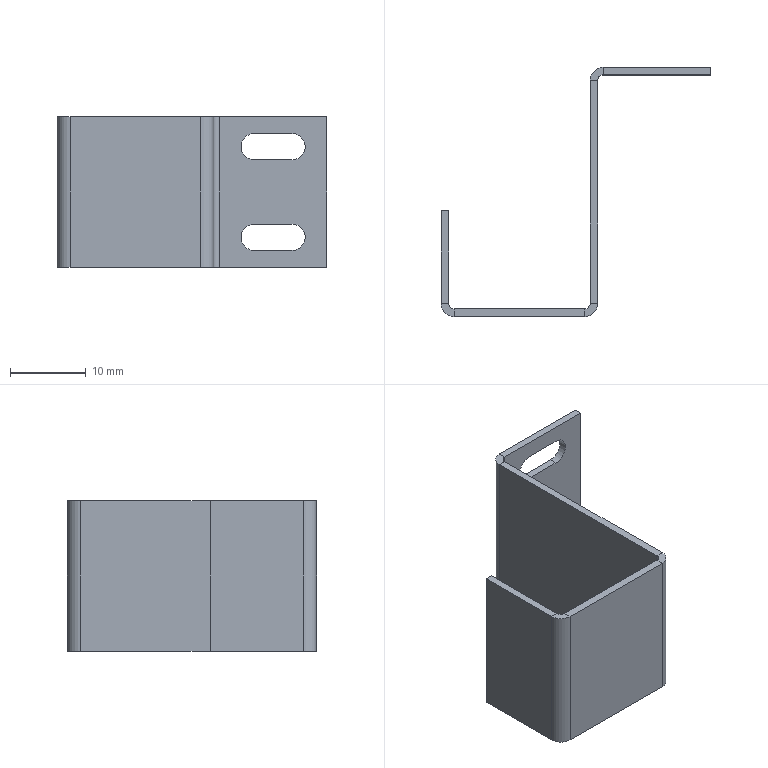Part | STEP file | PN_0038 | 1 solid | 38 faces | box 35.75 x 33 x 20 mm | volume 1529 mm3 | plane 28 | cylinder 10 | commonest cylinder face diameters 3.5 x4 1.473 x3 3.473 x3